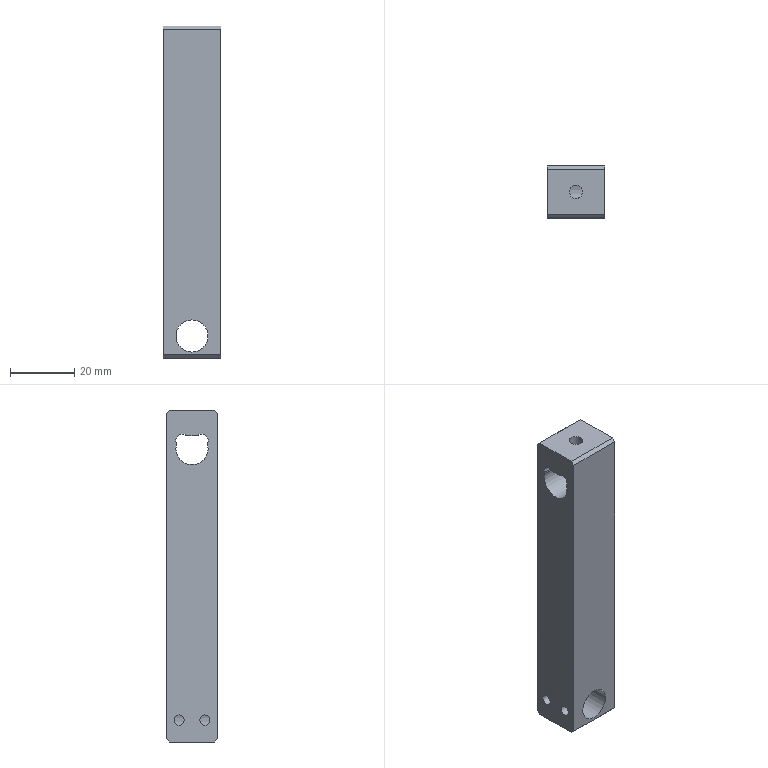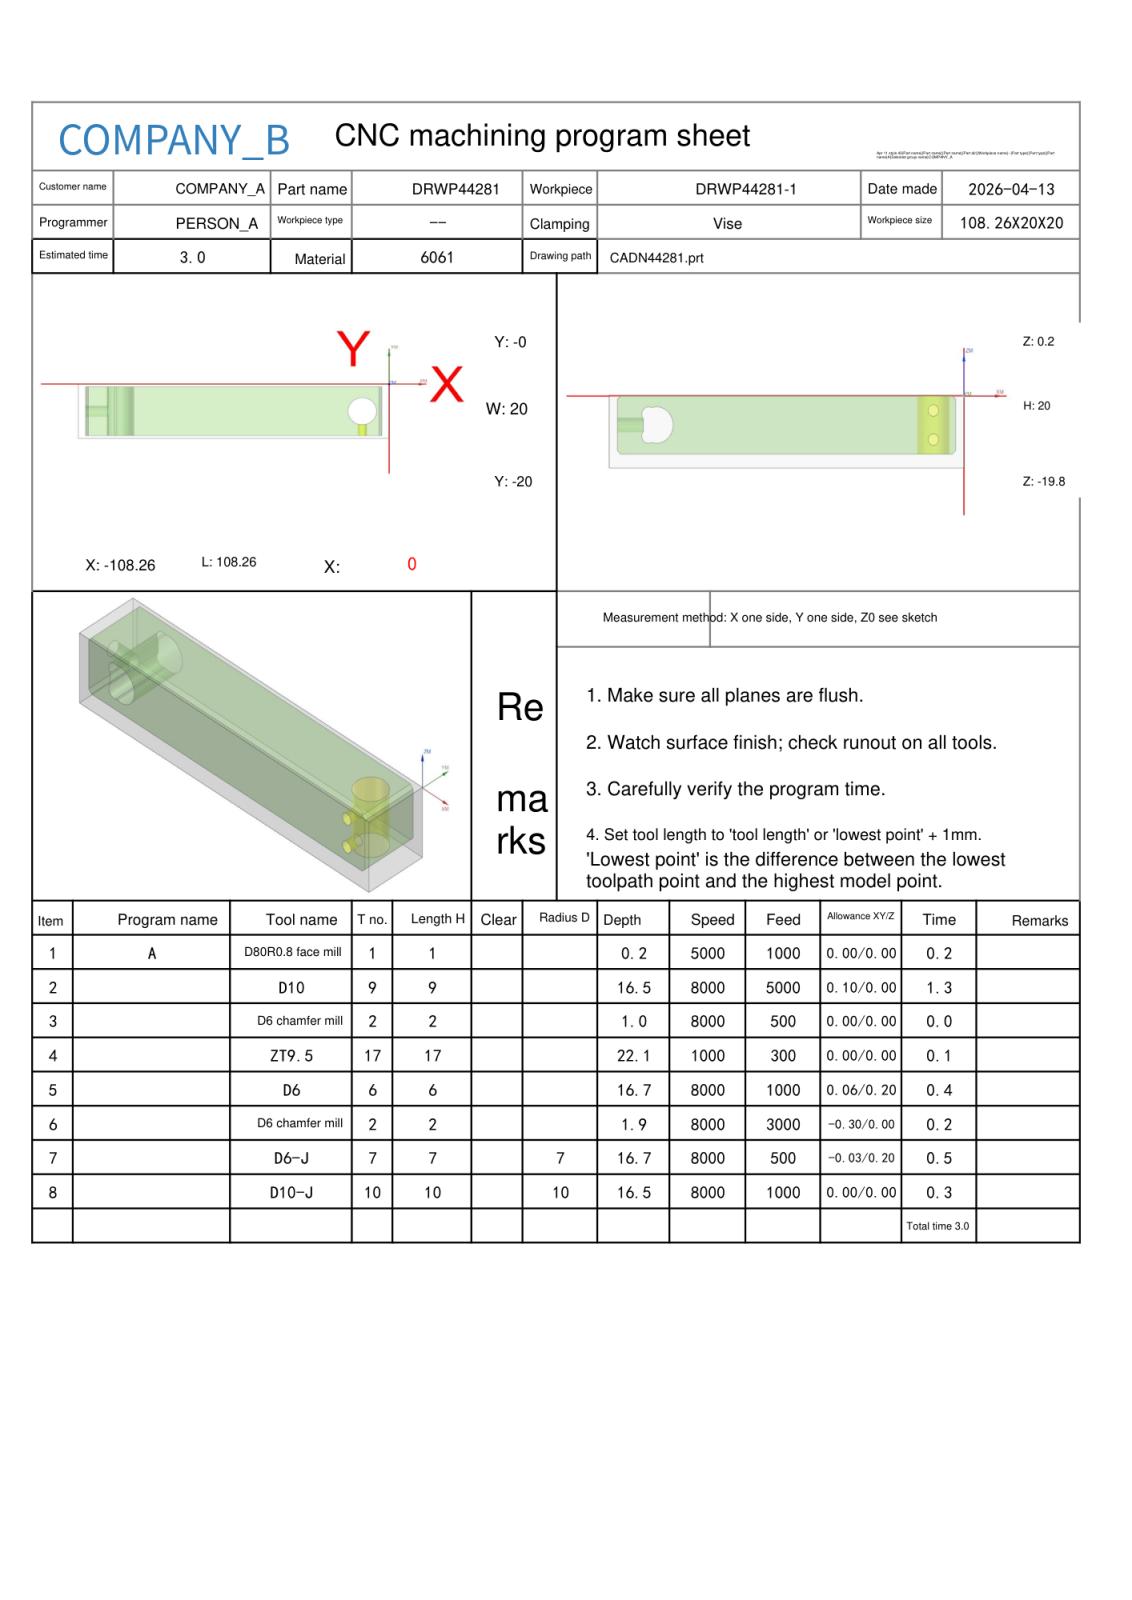NC program | NX | posted by the shop | part box 18 x 16 x 103.264 mm
Whole program:
%
O0001
(Machine time: 4.58 MIN)
(===Total Tool:7===)
(T1=D80R0.8 face mill D=80.  R=0.8  D-  H01 Z=0.    )
(T9=D10     D=10.  R=0.   D-  H09 Z=-16.3 )
(T2=D6 chamfer mill   D=6.   R=0.   D-  H02 Z=-1.7  )
(T17=ZT9.5  D=9.5  DR_a=118 D-  H17 Z=-21.85)
(T6=D6      D=6.   R=0.   D-  H06 Z=-16.5 )
(T7=D6-J    D=6.   R=0.   D7  H07 Z=-16.5 )
(T10=D10-J  D=10.  R=0.   D10 H10 Z=-16.3 )
G80 G90 G17 G49 G40
G91 G28 Z0
M01
N1 T01 M06
(D80R0.8 face mill D=80. R=0.8 H=01 ce=0.00 di=0.00)
G00 G90 G54 X42.5 Y-10. M03 S5000
G43 H01 Z20.
M08
Z2.
G01 Z0.0 F1000.
X37.5
X-145.764
X-150.764
Z2.
G00 Z20.
G91 G28 Z0.0
M05
M09
G91 G28 Z0.0
M01
N2 T09 M06
(D10  D=10. R=0. H=09 ce=0.10 di=0.00)
G00 G90 G54 X-54.132 Y4.1 M03 S8000
G43 H09 Z20.
M08
Z.5
G01 X-2.5 Z.356 F5000.
G02 X2.6 Y-1. Z.334 I0.0 J-5.1
G01 Y-19. Z.284
G02 X-2.5 Y-24.1 Z.262 I-5.1 J0.0
G01 X-105.764 Z-.025
G02 X-110.864 Y-19. Z-.048 I0.0 J5.1
G01 Y-1. Z-.098
G02 X-105.764 Y4.1 Z-.12 I5.1 J0.0
G01 X-2.5 Z-.407
G02 X2.6 Y-1. Z-.43 I0.0 J-5.1
G01 Y-19. Z-.48
G02 X-2.5 Y-24.1 Z-.502 I-5.1 J0.0
G01 X-105.764 Z-.789
G02 X-110.864 Y-19. Z-.811 I0.0 J5.1
G01 Y-1. Z-.861
G02 X-105.764 Y4.1 Z-.884 I5.1 J0.0
G01 X-2.5 Z-1.171
G02 X2.6 Y-1. Z-1.193 I0.0 J-5.1
G01 Y-19. Z-1.243
G02 X-2.5 Y-24.1 Z-1.265 I-5.1 J0.0
G01 X-105.764 Z-1.553
G02 X-110.864 Y-19. Z-1.575 I0.0 J5.1
G01 Y-1. Z-1.625
G02 X-105.764 Y4.1 Z-1.647 I5.1 J0.0
G01 X-2.5 Z-1.935
G02 X2.6 Y-1. Z-1.957 I0.0 J-5.1
G01 Y-19. Z-2.007
G02 X-2.5 Y-24.1 Z-2.029 I-5.1 J0.0
G01 X-105.764 Z-2.316
G02 X-110.864 Y-19. Z-2.339 I0.0 J5.1
G01 Y-1. Z-2.389
G02 X-105.764 Y4.1 Z-2.411 I5.1 J0.0
G01 X-2.5 Z-2.698
G02 X2.6 Y-1. Z-2.72 I0.0 J-5.1
G01 Y-19. Z-2.77
G02 X-2.5 Y-24.1 Z-2.793 I-5.1 J0.0
G01 X-105.764 Z-3.08
G02 X-110.864 Y-19. Z-3.102 I0.0 J5.1
G01 Y-1. Z-3.152
G02 X-105.764 Y4.1 Z-3.175 I5.1 J0.0
G01 X-2.5 Z-3.462
G02 X2.6 Y-1. Z-3.484 I0.0 J-5.1
G01 Y-19. Z-3.534
G02 X-2.5 Y-24.1 Z-3.556 I-5.1 J0.0
G01 X-105.764 Z-3.844
G02 X-110.864 Y-19. Z-3.866 I0.0 J5.1
G01 Y-1. Z-3.916
G02 X-105.764 Y4.1 Z-3.938 I5.1 J0.0
G01 X-2.5 Z-4.225
G02 X2.6 Y-1. Z-4.248 I0.0 J-5.1
G01 Y-19. Z-4.298
G02 X-2.5 Y-24.1 Z-4.32 I-5.1 J0.0
G01 X-105.764 Z-4.607
G02 X-110.864 Y-19. Z-4.63 I0.0 J5.1
G01 Y-1. Z-4.68
G02 X-105.764 Y4.1 Z-4.702 I5.1 J0.0
G01 X-2.5 Z-4.989
G02 X2.6 Y-1. Z-5.011 I0.0 J-5.1
G01 Y-19. Z-5.061
G02 X-2.5 Y-24.1 Z-5.084 I-5.1 J0.0
G01 X-105.764 Z-5.371
G02 X-110.864 Y-19. Z-5.393 I0.0 J5.1
G01 Y-1. Z-5.443
G02 X-105.764 Y4.1 Z-5.465 I5.1 J0.0
G01 X-2.5 Z-5.753
G02 X2.6 Y-1. Z-5.775 I0.0 J-5.1
G01 Y-19. Z-5.825
G02 X-2.5 Y-24.1 Z-5.847 I-5.1 J0.0
G01 X-105.764 Z-6.135
G02 X-110.864 Y-19. Z-6.157 I0.0 J5.1
G01 Y-1. Z-6.207
G02 X-105.764 Y4.1 Z-6.229 I5.1 J0.0
G01 X-2.5 Z-6.516
G02 X2.6 Y-1. Z-6.539 I0.0 J-5.1
G01 Y-19. Z-6.589
G02 X-2.5 Y-24.1 Z-6.611 I-5.1 J0.0
G01 X-105.764 Z-6.898
G02 X-110.864 Y-19. Z-6.92 I0.0 J5.1
G01 Y-1. Z-6.97
G02 X-105.764 Y4.1 Z-6.993 I5.1 J0.0
G01 X-2.5 Z-7.28
G02 X2.6 Y-1. Z-7.302 I0.0 J-5.1
G01 Y-19. Z-7.352
G02 X-2.5 Y-24.1 Z-7.375 I-5.1 J0.0
G01 X-105.764 Z-7.662
G02 X-110.864 Y-19. Z-7.684 I0.0 J5.1
G01 Y-1. Z-7.734
G02 X-105.764 Y4.1 Z-7.756 I5.1 J0.0
G01 X-2.5 Z-8.044
G02 X2.6 Y-1. Z-8.066 I0.0 J-5.1
G01 Y-19. Z-8.116
G02 X-2.5 Y-24.1 Z-8.138 I-5.1 J0.0
G01 X-105.764 Z-8.425
G02 X-110.864 Y-19. Z-8.448 I0.0 J5.1
G01 Y-1. Z-8.498
G02 X-105.764 Y4.1 Z-8.52 I5.1 J0.0
G01 X-2.5 Z-8.807
G02 X2.6 Y-1. Z-8.83 I0.0 J-5.1
G01 Y-19. Z-8.88
G02 X-2.5 Y-24.1 Z-8.902 I-5.1 J0.0
G01 X-105.764 Z-9.189
G02 X-110.864 Y-19. Z-9.211 I0.0 J5.1
G01 Y-1. Z-9.261
G02 X-105.764 Y4.1 Z-9.284 I5.1 J0.0
G01 X-2.5 Z-9.571
G02 X2.6 Y-1. Z-9.593 I0.0 J-5.1
G01 Y-19. Z-9.643
G02 X-2.5 Y-24.1 Z-9.665 I-5.1 J0.0
G01 X-105.764 Z-9.953
G02 X-110.864 Y-19. Z-9.975 I0.0 J5.1
G01 Y-1. Z-10.025
G02 X-105.764 Y4.1 Z-10.047 I5.1 J0.0
G01 X-2.5 Z-10.335
G02 X2.6 Y-1. Z-10.357 I0.0 J-5.1
G01 Y-19. Z-10.407
G02 X-2.5 Y-24.1 Z-10.429 I-5.1 J0.0
G01 X-105.764 Z-10.716
G02 X-110.864 Y-19. Z-10.739 I0.0 J5.1
G01 Y-1. Z-10.789
G02 X-105.764 Y4.1 Z-10.811 I5.1 J0.0
G01 X-2.5 Z-11.098
G02 X2.6 Y-1. Z-11.12 I0.0 J-5.1
G01 Y-19. Z-11.17
G02 X-2.5 Y-24.1 Z-11.193 I-5.1 J0.0
G01 X-105.764 Z-11.48
G02 X-110.864 Y-19. Z-11.502 I0.0 J5.1
G01 Y-1. Z-11.552
G02 X-105.764 Y4.1 Z-11.575 I5.1 J0.0
G01 X-2.5 Z-11.862
G02 X2.6 Y-1. Z-11.884 I0.0 J-5.1
G01 Y-19. Z-11.934
G02 X-2.5 Y-24.1 Z-11.956 I-5.1 J0.0
G01 X-105.764 Z-12.244
G02 X-110.864 Y-19. Z-12.266 I0.0 J5.1
G01 Y-1. Z-12.316
G02 X-105.764 Y4.1 Z-12.338 I5.1 J0.0
G01 X-2.5 Z-12.625
G02 X2.6 Y-1. Z-12.648 I0.0 J-5.1
G01 Y-19. Z-12.698
G02 X-2.5 Y-24.1 Z-12.72 I-5.1 J0.0
G01 X-105.764 Z-13.007
G02 X-110.864 Y-19. Z-13.03 I0.0 J5.1
G01 Y-1. Z-13.08
G02 X-105.764 Y4.1 Z-13.102 I5.1 J0.0
G01 X-2.5 Z-13.389
G02 X2.6 Y-1. Z-13.411 I0.0 J-5.1
G01 Y-19. Z-13.461
G02 X-2.5 Y-24.1 Z-13.484 I-5.1 J0.0
G01 X-105.764 Z-13.771
G02 X-110.864 Y-19. Z-13.793 I0.0 J5.1
G01 Y-1. Z-13.843
G02 X-105.764 Y4.1 Z-13.865 I5.1 J0.0
G01 X-2.5 Z-14.153
G02 X2.6 Y-1. Z-14.175 I0.0 J-5.1
G01 Y-19. Z-14.225
G02 X-2.5 Y-24.1 Z-14.247 I-5.1 J0.0
G01 X-105.764 Z-14.535
G02 X-110.864 Y-19. Z-14.557 I0.0 J5.1
G01 Y-1. Z-14.607
G02 X-105.764 Y4.1 Z-14.629 I5.1 J0.0
G01 X-2.5 Z-14.916
G02 X2.6 Y-1. Z-14.939 I0.0 J-5.1
G01 Y-19. Z-14.989
G02 X-2.5 Y-24.1 Z-15.011 I-5.1 J0.0
G01 X-105.764 Z-15.298
G02 X-110.864 Y-19. Z-15.32 I0.0 J5.1
G01 Y-1. Z-15.37
G02 X-105.764 Y4.1 Z-15.393 I5.1 J0.0
G01 X-2.5 Z-15.68
G02 X2.6 Y-1. Z-15.702 I0.0 J-5.1
G01 Y-19. Z-15.752
G02 X-2.5 Y-24.1 Z-15.775 I-5.1 J0.0
G01 X-105.764 Z-16.062
G02 X-110.864 Y-19. Z-16.084 I0.0 J5.1
G01 Y-1. Z-16.134
G02 X-105.764 Y4.1 Z-16.156 I5.1 J0.0
G01 X-54.132 Z-16.3
X-2.5
G02 X2.6 Y-1. I0.0 J-5.1
G01 Y-19.
G02 X-2.5 Y-24.1 I-5.1 J0.0
G01 X-105.764
G02 X-110.864 Y-19. I0.0 J5.1
G01 Y-1.
G02 X-105.764 Y4.1 I5.1 J0.0
G01 X-54.132
X-53.632
Z-15.3
G00 Z20.
G91 G28 Z0.0
M05
M09
G91 G28 Z0.0
M01
N3 T02 M06
(D6 chamfer mill  D=6. R=0. H=02 ce=0.00 di=0.00)
G00 G90 G54 X-9.334 Y-10. M03 S8000
G43 H02 Z20.
M08
G98 G81 X-9.334 Y-10. Z-.8 R1. F500.
G80
G00 Z20.
G91 G28 Z0.0
M05
M09
G91 G28 Z0.0
M01
N4 T17 M06
(ZT9.5 D=9.5 DR_a=118 H=17)
G00 G90 G54 X-9.334 Y-10. M03 S1000
G43 H17 Z20.
M08
G98 G83 X-9.334 Y-10. Z-21.854 R1. F300. Q2.
G80
G00 Z20.
G91 G28 Z0.0
M05
M09
G91 G28 Z0.0
M01
N5 T06 M06
(D6  D=6. R=0. H=06 ce=0.06 di=0.20)
G00 G90 G54 X-9.334 Y-10. M03 S8000
G43 H06 Z20.
M08
Z.5
G03 X-8.364 Y-9.03 I0.0 J.97 F1000.
X-9.334 Y-8.06 I-.97 J0.0
X-9.334 Y-8.06 Z0.0 I0.0 J-1.94
X-9.334 Y-8.06 Z-.5 I0.0 J-1.94
X-9.334 Y-8.06 Z-1. I0.0 J-1.94
X-9.334 Y-8.06 Z-1.5 I0.0 J-1.94
X-9.334 Y-8.06 Z-2. I0.0 J-1.94
X-9.334 Y-8.06 Z-2.5 I0.0 J-1.94
X-9.334 Y-8.06 Z-3. I0.0 J-1.94
X-9.334 Y-8.06 Z-3.5 I0.0 J-1.94
X-9.334 Y-8.06 Z-4. I0.0 J-1.94
X-9.334 Y-8.06 Z-4.5 I0.0 J-1.94
X-9.334 Y-8.06 Z-5. I0.0 J-1.94
X-9.334 Y-8.06 Z-5.5 I0.0 J-1.94
X-9.334 Y-8.06 Z-6. I0.0 J-1.94
X-9.334 Y-8.06 Z-6.5 I0.0 J-1.94
X-9.334 Y-8.06 Z-7. I0.0 J-1.94
X-9.334 Y-8.06 Z-7.5 I0.0 J-1.94
X-9.334 Y-8.06 Z-8. I0.0 J-1.94
X-9.334 Y-8.06 Z-8.5 I0.0 J-1.94
X-9.334 Y-8.06 Z-9. I0.0 J-1.94
X-9.334 Y-8.06 Z-9.5 I0.0 J-1.94
X-9.334 Y-8.06 Z-10. I0.0 J-1.94
X-9.334 Y-8.06 Z-10.5 I0.0 J-1.94
X-9.334 Y-8.06 Z-11. I0.0 J-1.94
X-9.334 Y-8.06 Z-11.5 I0.0 J-1.94
X-9.334 Y-8.06 Z-12. I0.0 J-1.94
X-9.334 Y-8.06 Z-12.5 I0.0 J-1.94
X-9.334 Y-8.06 Z-13. I0.0 J-1.94
X-9.334 Y-8.06 Z-13.5 I0.0 J-1.94
X-9.334 Y-8.06 Z-14. I0.0 J-1.94
X-9.334 Y-8.06 Z-14.5 I0.0 J-1.94
X-9.334 Y-8.06 Z-15. I0.0 J-1.94
X-9.334 Y-8.06 Z-15.5 I0.0 J-1.94
X-9.334 Y-8.06 Z-16. I0.0 J-1.94
X-9.334 Y-8.06 Z-16.5 I0.0 J-1.94
X-11.274 Y-10. I0.0 J-1.94
X-9.334 Y-11.94 I1.94 J0.0
X-7.394 Y-10. I0.0 J1.94
X-9.334 Y-8.06 I-1.94 J0.0
X-10.304 Y-9.03 I0.0 J-.97
X-9.334 Y-10. I.97 J0.0
G00 Z20.
G91 G28 Z0.0
M05
M09
G91 G28 Z0.0
M01
N6 T02 M06
(D6 chamfer mill  D=6. R=0. H=02 ce=0.00 di=0.00)
G00 G90 G54 X-3.039 Y-20.207 M03 S8000
G43 H02 Z20.
M08
Z2.935
G01 Z-1.499 F3000.
X-3.211 Y-20.267
X-3.5 Y-20.3
X-104.764
X-105.054 Y-20.267
X-105.225 Y-20.207
Z2.935
G00 Z20.
Y.207
Z2.935
G01 Z-1.499
X-105.054 Y.267
X-104.764 Y.3
X-54.132
X-3.5
X-3.211 Y.267
X-3.039 Y.207
Z2.935
G00 Z20.
G00 G90 X-10.634 Y-7. M03 S8000
Z20.
Z-.5
G01 Z-1. F500.
G03 X-13.634 Y-10. I0.0 J-3.
X-9.334 Y-14.3 I4.3 J0.0
X-5.034 Y-10. I0.0 J4.3
X-9.334 Y-5.7 I-4.3 J0.0
X-13.634 Y-10. I0.0 J-4.3
X-10.634 Y-13. I3. J0.0
G01 Z-.5
G00 Z20.
G00 G90 X-106.472 Y-21.9 M03 S6500
Z20.
Z-.2
G01 Z-1.7 F1500.
X-106.463 Y-21.832
X-106.464 Y-21.763
Y1.763
X-106.463 Y1.832
X-106.472 Y1.9
Z-.2
G00 Z20.
X-1.792
Z-.2
G01 Z-1.7
X-1.801 Y1.832
X-1.8 Y1.763
Y-21.763
X-1.801 Y-21.832
X-1.792 Y-21.9
Z-.2
G00 Z20.
G91 G28 Z0.0
M05
M09
G91 G28 Z0.0
M01
N7 T07 M06
(D6-J  D=6. R=0. H=07 ce=-0.03 di=0.20)
G00 G90 G54 X-9.334 Y-10. M03 S8000
G43 H07 Z20.
M08
Z.5
G41 D07
G01 X-9.138 Y-9.961 F500.
G03 X-8.329 Y-8.975 I-.196 J.986
X-9.334 Y-7.97 I-1.005 J0.0
X-9.334 Y-7.97 Z-.5 I0.0 J-2.03
X-9.334 Y-7.97 Z-1.5 I0.0 J-2.03
X-9.334 Y-7.97 Z-2.5 I0.0 J-2.03
X-9.334 Y-7.97 Z-3.5 I0.0 J-2.03
X-9.334 Y-7.97 Z-4.5 I0.0 J-2.03
X-9.334 Y-7.97 Z-5.5 I0.0 J-2.03
X-9.334 Y-7.97 Z-6.5 I0.0 J-2.03
X-9.334 Y-7.97 Z-7.5 I0.0 J-2.03
X-9.334 Y-7.97 Z-8.5 I0.0 J-2.03
X-9.334 Y-7.97 Z-9.5 I0.0 J-2.03
X-9.334 Y-7.97 Z-10.5 I0.0 J-2.03
X-9.334 Y-7.97 Z-11.5 I0.0 J-2.03
X-9.334 Y-7.97 Z-12.5 I0.0 J-2.03
X-9.334 Y-7.97 Z-13.5 I0.0 J-2.03
X-9.334 Y-7.97 Z-14.5 I0.0 J-2.03
X-9.334 Y-7.97 Z-15.5 I0.0 J-2.03
X-9.334 Y-7.97 Z-16.5 I0.0 J-2.03
X-11.364 Y-10. I0.0 J-2.03
X-9.334 Y-12.03 I2.03 J0.0
X-7.304 Y-10. I0.0 J2.03
X-9.334 Y-7.97 I-2.03 J0.0
X-10.339 Y-8.975 I0.0 J-1.005
X-9.53 Y-9.961 I1.005 J0.0
G01 G40 X-9.334 Y-10.
G00 Z20.
G91 G28 Z0.0
M05
M09
G91 G28 Z0.0
M01
N8 T10 M06
(D10-J  D=10. R=0. H=10 ce=0.00 di=0.00)
G00 G90 G54 X-106.777 Y5.116 M03 S8000
G43 H10 Z20.
M08
Z-15.8
G01 Z-16.3 F1000.
G41 D10
X-106.761 Y4.917
G03 X-105.764 Y4. I.997 J.083
G01 X-2.5
G02 X2.5 Y-1. I0.0 J-5.
G01 Y-19.
G02 X-2.5 Y-24. I-5. J0.0
G01 X-105.764
G02 X-110.764 Y-19. I0.0 J5.
G01 Y-1.
G02 X-105.764 Y4. I5. J0.0
G01 X-105.264
G03 X-104.264 Y5. I0.0 J1.
G01 G40 Y5.2
Z-15.8
G00 Z20.
M05
M09
G91 G28 Z0.0
G91 G28 Y0.0
M30
%